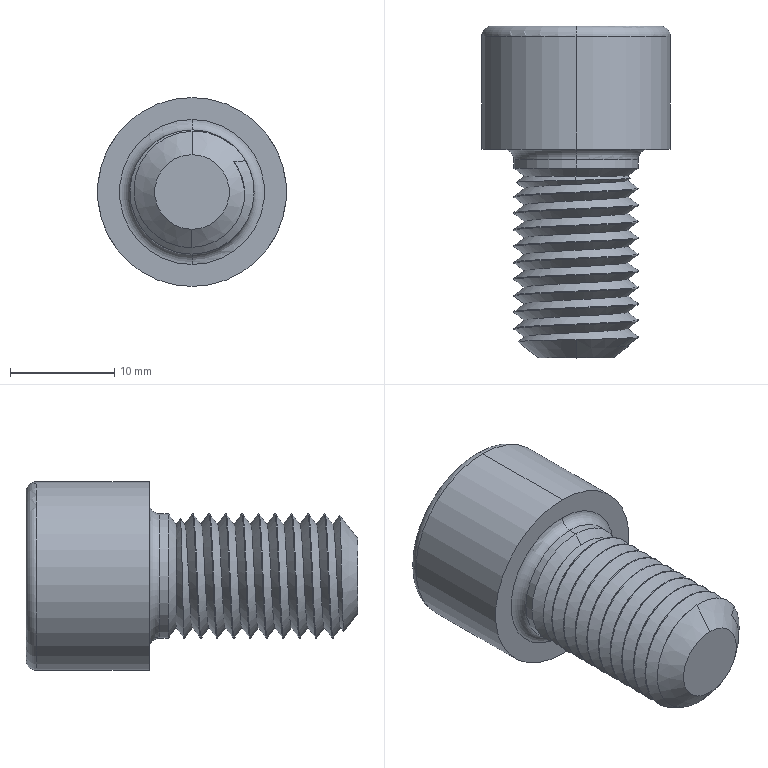Part | STEP file | Parafuso M12 - 20mm | 1 solid | 50 faces | box 18.1 x 31.8 x 18.1 mm | volume 4507 mm3 | cylinder 24 | plane 10 | cone 8 | torus 6 | spline 2 | commonest cylinder face diameters 11.9 x22 18.1 x2